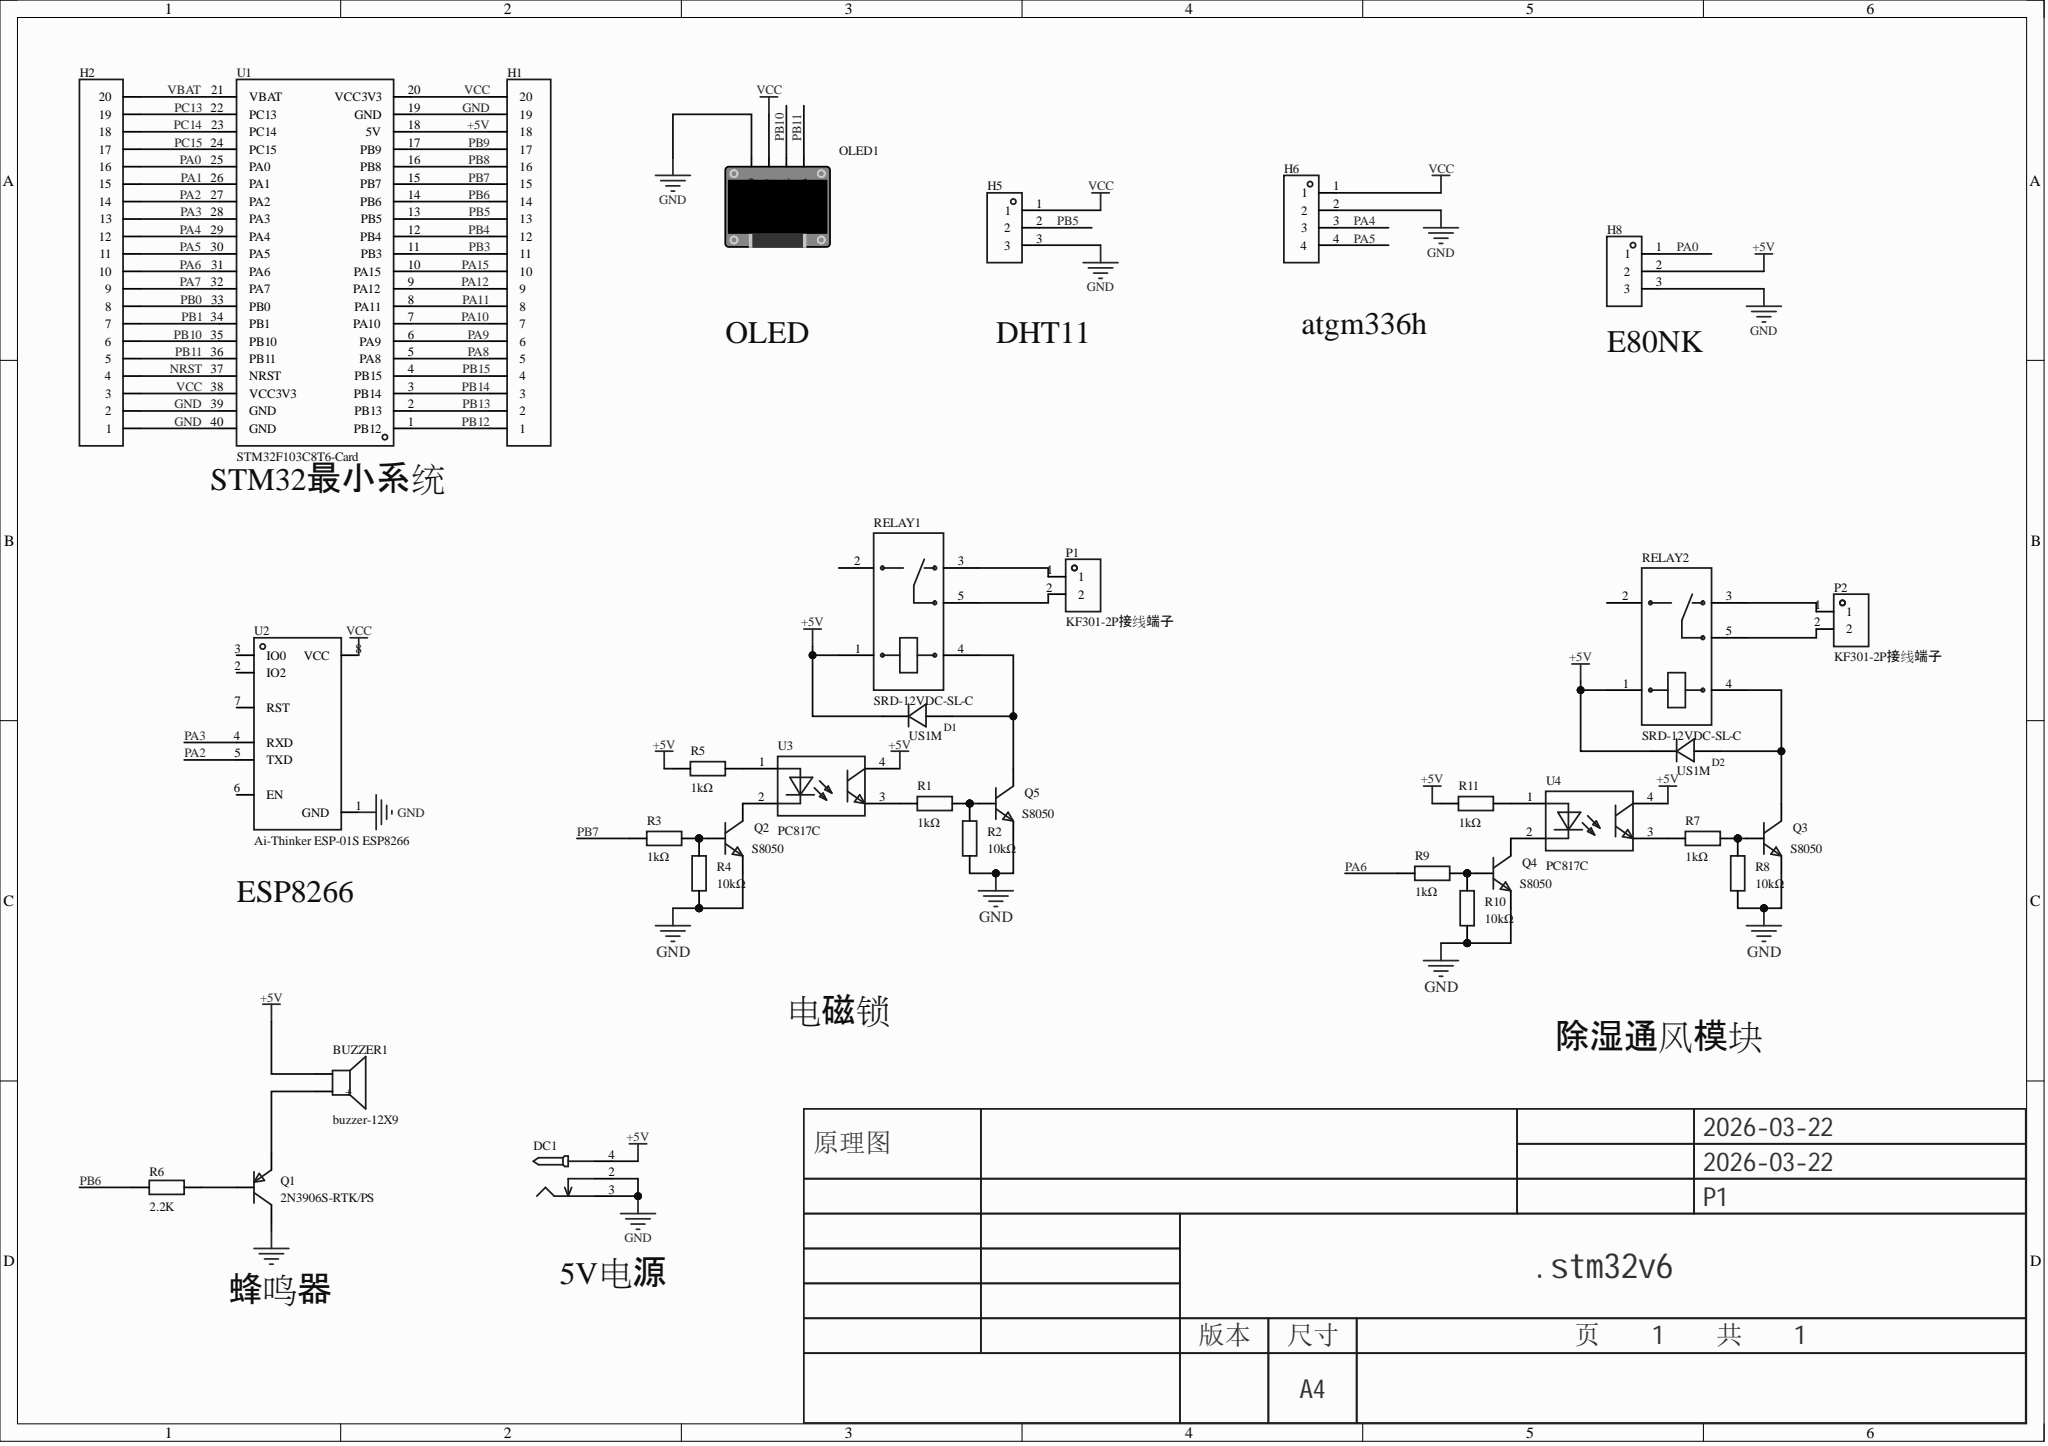Circuit board | Altium Designer | 34 parts | 55 nets
Bill of materials:
Comment,Description,Designator,Footprint,LibRef,Quantity
"buzzer-12X9","","BUZZER1","BUZ-TH_BD12.0-P7.60-D0.6-FD","buzzer-12X9","1"
"US1M","二极管配置:独立式;直流反向耐压(Vr):1kV;平均整流电流(Io):1A;正向压降(Vf):1.7V@1A;反向恢复时间(trr):75ns;","D1, D2","SMA_L4.4-W2.8-LS5.4-RD","US1M_C412437","2"
"","","DC1","DC-2.0","DC-005_2.0","1"
"","","H1, H2","HDR-TH_20P-P2.54-V-F","HDR-F_2.54_1x20P","2"
"","","H5","HDR-TH_3P-P2.54-V-F","HDR-F_2.54_1x3P","1"
"","","H6","HDR-TH_4P-P2.54-V-F","HDR-F_2.54_1x4P","1"
"","","H8","HDR-TH_3P-P2.54-V-M","HDR-M_2.54_1x3P","1"
"","","OLED1","0.96OLED_4P","0.96OLED模块_4P","1"
"KF301-2P接线端子","","P1, P2","CONN-TH_XY301V-A-5.0-2P","KF301-2P接线端子","2"
"2N3906S-RTK/PS","","Q1","SOT-23-3_L2.9-W1.3-P1.90-LS2.4-TR","2N3906S-RTK/PS","1"
"S8050","晶体管类型:NPN;集射极击穿电压(Vceo):25V;集电极电流(Ic):500mA;功率(Pd):300mW;直流电流增益(hFE@Ic,Vce):120@50mA,1V;","Q2, Q3, Q4, Q5","SOT-23-3_L2.9-W1.6-P1.90-LS2.8-BR","S8050_C105433","4"
"1kΩ","","R1, R3, R5, R7, R9, R11","R0603","0603WAF1001T5E","6"
"10kΩ","","R2, R4, R8, R10","R0603","0603WAF1002T5E","4"
"2.2K","","R6","R0805","Res_0805","1"
"SRD-12VDC-SL-C","线圈电压:12V;引脚数:5;触点形式:一组转换:1C(单刀双掷-转换);触点容量(电阻负载):-;","RELAY1, RELAY2","RELAY-TH_SRD-XXVDC-XL-C","SRD-12VDC-SL-C","2"
"STM32F103C8T6-Card","","U1","CONN-TH_L53.3-W22.9_STM32F103C8T6-CARD","STM32F103C8T6-Card","1"
"Ai-Thinker ESP-01S ESP8266","","U2","WIFIM-TH_8P-L24.7-W14.4-P2.54","Ai-Thinker ESP-01S ESP8266","1"
"PC817C","","U3, U4","OPTO-SMD-4_L4.6-W6.5-P2.54-LS10.3-TL","PC817C_C3025164","2"
Netlist (Protel format):
[
BUZZER1
BUZ-TH_BD12.0-P7.60-D0.6-FD
buzzer-12X9



]
[
D1
SMA_L4.4-W2.8-LS5.4-RD
US1M



]
[
D2
SMA_L4.4-W2.8-LS5.4-RD
US1M



]
[
DC1
DC-2.0




]
[
H1
HDR-TH_20P-P2.54-V-F




]
[
H2
HDR-TH_20P-P2.54-V-F




]
[
H5
HDR-TH_3P-P2.54-V-F




]
[
H6
HDR-TH_4P-P2.54-V-F




]
[
H8
HDR-TH_3P-P2.54-V-M




]
[
OLED1
0.96OLED_4P




]
[
P1
CONN-TH_XY301V-A-5.0-2P
KF301-2P接线端子



]
[
P2
CONN-TH_XY301V-A-5.0-2P
KF301-2P接线端子



]
[
Q1
SOT-23-3_L2.9-W1.3-P1.90-LS2.4-TR
2N3906S-RTK/PS



]
[
Q2
SOT-23-3_L2.9-W1.6-P1.90-LS2.8-BR
S8050



]
[
Q3
SOT-23-3_L2.9-W1.6-P1.90-LS2.8-BR
S8050



]
[
Q4
SOT-23-3_L2.9-W1.6-P1.90-LS2.8-BR
S8050



]
[
Q5
SOT-23-3_L2.9-W1.6-P1.90-LS2.8-BR
S8050



]
[
R1
R0603
1kΩ



]
[
R2
R0603
10kΩ



]
[
R3
R0603
1kΩ



]
[
R4
R0603
10kΩ



]
[
R5
R0603
1kΩ



]
[
R6
R0805
2.2K



]
[
R7
R0603
1kΩ



]
[
R8
R0603
10kΩ



]
[
R9
R0603
1kΩ



]
[
R10
R0603
10kΩ



]
[
R11
R0603
1kΩ



]
[
RELAY1
RELAY-TH_SRD-XXVDC-XL-C
SRD-12VDC-SL-C



]
[
RELAY2
RELAY-TH_SRD-XXVDC-XL-C
SRD-12VDC-SL-C



]
[
U1
CONN-TH_L53.3-W22.9_STM32F103C8T6-CARD
STM32F103C8T6-Card



]
[
U2
WIFIM-TH_8P-L24.7-W14.4-P2.54
Ai-Thinker ESP-01S ESP8266



]
[
U3
OPTO-SMD-4_L4.6-W6.5-P2.54-LS10.3-TL
PC817C



]
[
U4
OPTO-SMD-4_L4.6-W6.5-P2.54-LS10.3-TL
PC817C



]
(
VCC
H1-20
H2-3
H5-1
H6-1
OLED1-2
U1-20
U1-38
U2-8
)
(
VBAT
H2-20
U1-21
)
(
PC15
H2-17
U1-24
)
(
PC14
H2-18
U1-23
)
(
PC13
H2-19
U1-22
)
(
PB15
H1-4
U1-4
)
(
PB14
H1-3
U1-3
)
(
PB13
H1-2
U1-2
)
(
PB12
H1-1
U1-1
)
(
PB11
H2-5
OLED1-4
U1-36
)
(
PB10
H2-6
OLED1-3
U1-35
)
(
PB9
H1-17
U1-17
)
(
PB8
H1-16
U1-16
)
(
PB7
H1-15
R3-1
U1-15
)
(
PB6
H1-14
R6-1
U1-14
)
(
PB5
H1-13
H5-2
U1-13
)
(
PB4
H1-12
U1-12
)
(
PB3
H1-11
U1-11
)
(
PB1
H2-7
U1-34
)
(
PB0
H2-8
U1-33
)
(
PA15
H1-10
U1-10
)
(
PA12
H1-9
U1-9
)
(
PA11
H1-8
U1-8
)
(
PA10
H1-7
U1-7
)
(
PA9
H1-6
U1-6
)
(
PA8
H1-5
U1-5
)
(
PA7
H2-9
U1-32
)
(
PA6
H2-10
R9-1
U1-31
)
(
PA5
H2-11
H6-4
U1-30
)
(
PA4
H2-12
H6-3
U1-29
)
(
PA3
H2-13
U1-28
U2-4
)
(
PA2
H2-14
U1-27
U2-5
)
(
PA1
H2-15
U1-26
)
(
PA0
H2-16
H8-1
U1-25
)
(
NRST
H2-4
U1-37
)
(
NetR11_2
R11-2
U4-1
)
(
NetR7_1
R7-1
U4-3
)
(
NetR5_2
R5-2
U3-1
)
(
NetR1_1
R1-1
U3-3
)
(
NetQ5_1
Q5-1
R1-2
R2-2
)
(
NetQ4_3
Q4-3
U4-2
)
(
NetQ4_1
Q4-1
R9-2
R10-2
)
(
NetQ3_1
Q3-1
R7-2
R8-2
)
(
NetQ2_3
Q2-3
U3-2
)
(
NetQ2_1
Q2-1
R3-2
R4-2
)
(
NetQ1_2
Q1-2
R6-2
)
(
NetP2_2
P2-2
RELAY2-5
)
(
NetP2_1
P2-1
RELAY2-3
)
(
NetP1_2
P1-2
RELAY1-5
)
(
NetP1_1
P1-1
RELAY1-3
)
(
NetD2_2
D2-2
Q3-3
RELAY2-4
)
(
NetD1_2
D1-2
Q5-3
RELAY1-4
)
(
NetBUZZER1_1
BUZZER1-1
Q1-1
)
(
GND
DC1-2
DC1-3
H1-19
H2-1
H2-2
H5-3
H6-2
H8-3
OLED1-1
Q1-3
Q2-2
Q3-2
Q4-2
Q5-2
R2-1
R4-1
R8-1
R10-1
U1-19
U1-39
U1-40
U2-1
)
(
+5V
BUZZER1-2
D1-1
D2-1
DC1-4
H1-18
H8-2
R5-1
R11-1
RELAY1-1
RELAY2-1
U1-18
U3-4
U4-4
)